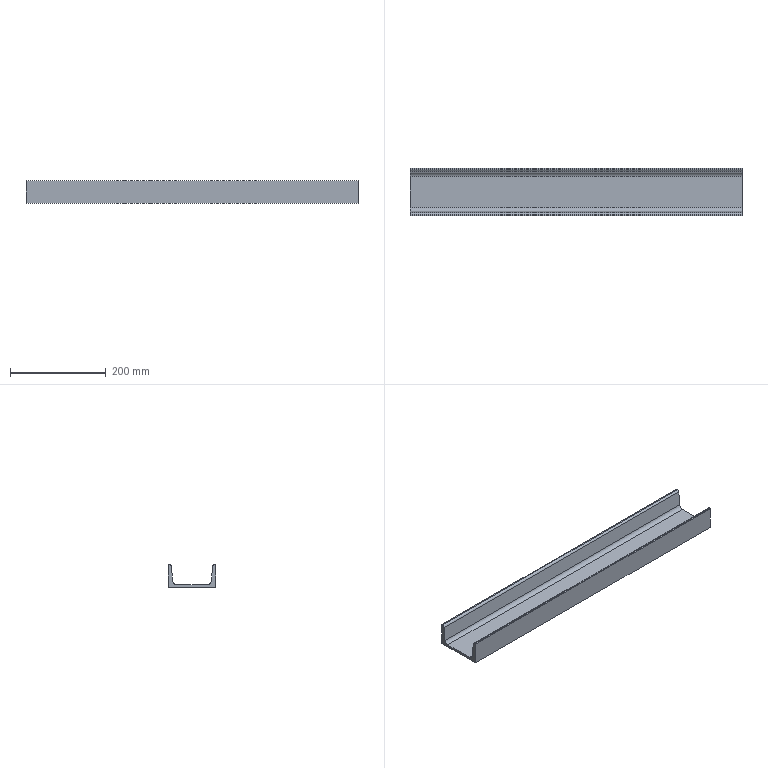Part | SolidWorks | features Fillet 2, Extrusion 1 | 1 solid | 14 faces | box 695 x 100 x 48 mm | volume 885612 mm3 | plane 10 | cylinder 4 | commonest cylinder face diameters 8.5 x2 17 x2
STEP:
#1=CARTESIAN_POINT('',(695.,43.252,44.173));
#2=VERTEX_POINT('',#1);
#3=CARTESIAN_POINT('',(695.,40.13,12.954));
#4=VERTEX_POINT('',#3);
#5=CARTESIAN_POINT('',(695.,39.365,5.3));
#6=DIRECTION('',(0.,-0.0995,-0.995));
#7=VECTOR('',#6,1000.);
#8=LINE('',#5,#7);
#9=EDGE_CURVE('',#2,#4,#8,.T.);
#10=ORIENTED_EDGE('',*,*,#9,.F.);
#11=CARTESIAN_POINT('',(0.,43.252,44.173));
#12=VERTEX_POINT('',#11);
#13=CARTESIAN_POINT('',(695.,43.252,44.173));
#14=DIRECTION('',(-1.,0.,0.));
#15=VECTOR('',#14,1000.);
#16=LINE('',#13,#15);
#17=EDGE_CURVE('',#2,#12,#16,.T.);
#18=ORIENTED_EDGE('',*,*,#17,.T.);
#19=CARTESIAN_POINT('',(0.,40.13,12.954));
#20=VERTEX_POINT('',#19);
#21=CARTESIAN_POINT('',(0.,39.365,5.3));
#22=DIRECTION('',(0.,-0.0995,-0.995));
#23=VECTOR('',#22,1000.);
#24=LINE('',#21,#23);
#25=EDGE_CURVE('',#12,#20,#24,.T.);
#26=ORIENTED_EDGE('',*,*,#25,.T.);
#27=CARTESIAN_POINT('',(695.,40.13,12.954));
#28=DIRECTION('',(1.,0.,0.));
#29=VECTOR('',#28,1000.);
#30=LINE('',#27,#29);
#31=EDGE_CURVE('',#20,#4,#30,.T.);
#32=ORIENTED_EDGE('',*,*,#31,.T.);
#33=EDGE_LOOP('',(#10,#18,#26,#32));
#34=FACE_OUTER_BOUND('',#33,.T.);
#35=CARTESIAN_POINT('',(695.,39.365,5.3));
#36=DIRECTION('',(0.,0.995,-0.0995));
#37=DIRECTION('',(0.,0.0995,0.995));
#38=AXIS2_PLACEMENT_3D('',#35,#36,#37);
#39=PLANE('',#38);
#40=ADVANCED_FACE('',(#34),#39,.F.);
#41=CARTESIAN_POINT('',(0.,31.673,5.3));
#42=VERTEX_POINT('',#41);
#43=CARTESIAN_POINT('',(0.,-31.673,5.3));
#44=VERTEX_POINT('',#43);
#45=CARTESIAN_POINT('',(0.,-39.365,5.3));
#46=DIRECTION('',(0.,-1.,0.));
#47=VECTOR('',#46,1000.);
#48=LINE('',#45,#47);
#49=EDGE_CURVE('',#42,#44,#48,.T.);
#50=ORIENTED_EDGE('',*,*,#49,.T.);
#51=CARTESIAN_POINT('',(695.,-31.673,5.3));
#52=VERTEX_POINT('',#51);
#53=CARTESIAN_POINT('',(695.,-31.673,5.3));
#54=DIRECTION('',(1.,0.,0.));
#55=VECTOR('',#54,1000.);
#56=LINE('',#53,#55);
#57=EDGE_CURVE('',#44,#52,#56,.T.);
#58=ORIENTED_EDGE('',*,*,#57,.T.);
#59=CARTESIAN_POINT('',(695.,31.673,5.3));
#60=VERTEX_POINT('',#59);
#61=CARTESIAN_POINT('',(695.,-39.365,5.3));
#62=DIRECTION('',(0.,-1.,0.));
#63=VECTOR('',#62,1000.);
#64=LINE('',#61,#63);
#65=EDGE_CURVE('',#60,#52,#64,.T.);
#66=ORIENTED_EDGE('',*,*,#65,.F.);
#67=CARTESIAN_POINT('',(0.,31.673,5.3));
#68=DIRECTION('',(-1.,0.,0.));
#69=VECTOR('',#68,1000.);
#70=LINE('',#67,#69);
#71=EDGE_CURVE('',#60,#42,#70,.T.);
#72=ORIENTED_EDGE('',*,*,#71,.T.);
#73=EDGE_LOOP('',(#50,#58,#66,#72));
#74=FACE_OUTER_BOUND('',#73,.T.);
#75=CARTESIAN_POINT('',(695.,-39.365,5.3));
#76=DIRECTION('',(0.,0.,-1.));
#77=DIRECTION('',(-1.,0.,0.));
#78=AXIS2_PLACEMENT_3D('',#75,#76,#77);
#79=PLANE('',#78);
#80=ADVANCED_FACE('',(#74),#79,.F.);
#81=CARTESIAN_POINT('',(0.,-40.13,12.954));
#82=VERTEX_POINT('',#81);
#83=CARTESIAN_POINT('',(0.,-43.252,44.173));
#84=VERTEX_POINT('',#83);
#85=CARTESIAN_POINT('',(0.,-39.365,5.3));
#86=DIRECTION('',(0.,-0.0995,0.995));
#87=VECTOR('',#86,1000.);
#88=LINE('',#85,#87);
#89=EDGE_CURVE('',#82,#84,#88,.T.);
#90=ORIENTED_EDGE('',*,*,#89,.T.);
#91=CARTESIAN_POINT('',(695.,-43.252,44.173));
#92=VERTEX_POINT('',#91);
#93=CARTESIAN_POINT('',(695.,-43.252,44.173));
#94=DIRECTION('',(1.,0.,0.));
#95=VECTOR('',#94,1000.);
#96=LINE('',#93,#95);
#97=EDGE_CURVE('',#84,#92,#96,.T.);
#98=ORIENTED_EDGE('',*,*,#97,.T.);
#99=CARTESIAN_POINT('',(695.,-40.13,12.954));
#100=VERTEX_POINT('',#99);
#101=CARTESIAN_POINT('',(695.,-39.365,5.3));
#102=DIRECTION('',(0.,-0.0995,0.995));
#103=VECTOR('',#102,1000.);
#104=LINE('',#101,#103);
#105=EDGE_CURVE('',#100,#92,#104,.T.);
#106=ORIENTED_EDGE('',*,*,#105,.F.);
#107=CARTESIAN_POINT('',(0.,-40.13,12.954));
#108=DIRECTION('',(-1.,0.,0.));
#109=VECTOR('',#108,1000.);
#110=LINE('',#107,#109);
#111=EDGE_CURVE('',#100,#82,#110,.T.);
#112=ORIENTED_EDGE('',*,*,#111,.T.);
#113=EDGE_LOOP('',(#90,#98,#106,#112));
#114=FACE_OUTER_BOUND('',#113,.T.);
#115=CARTESIAN_POINT('',(695.,-39.365,5.3));
#116=DIRECTION('',(0.,-0.995,-0.0995));
#117=DIRECTION('',(0.,0.0995,-0.995));
#118=AXIS2_PLACEMENT_3D('',#115,#116,#117);
#119=PLANE('',#118);
#120=ADVANCED_FACE('',(#114),#119,.F.);
#121=CARTESIAN_POINT('',(695.,-47.481,48.));
#122=VERTEX_POINT('',#121);
#123=CARTESIAN_POINT('',(695.,-50.,48.));
#124=VERTEX_POINT('',#123);
#125=CARTESIAN_POINT('',(695.,-43.635,48.));
#126=DIRECTION('',(0.,-1.,0.));
#127=VECTOR('',#126,1000.);
#128=LINE('',#125,#127);
#129=EDGE_CURVE('',#122,#124,#128,.T.);
#130=ORIENTED_EDGE('',*,*,#129,.F.);
#131=CARTESIAN_POINT('',(0.,-47.481,48.));
#132=VERTEX_POINT('',#131);
#133=CARTESIAN_POINT('',(695.,-47.481,48.));
#134=DIRECTION('',(-1.,0.,0.));
#135=VECTOR('',#134,1000.);
#136=LINE('',#133,#135);
#137=EDGE_CURVE('',#122,#132,#136,.T.);
#138=ORIENTED_EDGE('',*,*,#137,.T.);
#139=CARTESIAN_POINT('',(0.,-50.,48.));
#140=VERTEX_POINT('',#139);
#141=CARTESIAN_POINT('',(0.,-43.635,48.));
#142=DIRECTION('',(0.,-1.,0.));
#143=VECTOR('',#142,1000.);
#144=LINE('',#141,#143);
#145=EDGE_CURVE('',#132,#140,#144,.T.);
#146=ORIENTED_EDGE('',*,*,#145,.T.);
#147=CARTESIAN_POINT('',(695.,-50.,48.));
#148=DIRECTION('',(-1.,0.,0.));
#149=VECTOR('',#148,1000.);
#150=LINE('',#147,#149);
#151=EDGE_CURVE('',#124,#140,#150,.T.);
#152=ORIENTED_EDGE('',*,*,#151,.F.);
#153=EDGE_LOOP('',(#130,#138,#146,#152));
#154=FACE_OUTER_BOUND('',#153,.T.);
#155=CARTESIAN_POINT('',(695.,-43.635,48.));
#156=DIRECTION('',(0.,0.,-1.));
#157=DIRECTION('',(-1.,0.,0.));
#158=AXIS2_PLACEMENT_3D('',#155,#156,#157);
#159=PLANE('',#158);
#160=ADVANCED_FACE('',(#154),#159,.F.);
#161=CARTESIAN_POINT('',(0.,-50.,0.));
#162=VERTEX_POINT('',#161);
#163=CARTESIAN_POINT('',(0.,-50.,0.));
#164=DIRECTION('',(0.,0.,-1.));
#165=VECTOR('',#164,1000.);
#166=LINE('',#163,#165);
#167=EDGE_CURVE('',#140,#162,#166,.T.);
#168=ORIENTED_EDGE('',*,*,#167,.T.);
#169=CARTESIAN_POINT('',(695.,-50.,0.));
#170=VERTEX_POINT('',#169);
#171=CARTESIAN_POINT('',(695.,-50.,0.));
#172=DIRECTION('',(-1.,0.,0.));
#173=VECTOR('',#172,1000.);
#174=LINE('',#171,#173);
#175=EDGE_CURVE('',#170,#162,#174,.T.);
#176=ORIENTED_EDGE('',*,*,#175,.F.);
#177=CARTESIAN_POINT('',(695.,-50.,0.));
#178=DIRECTION('',(0.,0.,-1.));
#179=VECTOR('',#178,1000.);
#180=LINE('',#177,#179);
#181=EDGE_CURVE('',#124,#170,#180,.T.);
#182=ORIENTED_EDGE('',*,*,#181,.F.);
#183=ORIENTED_EDGE('',*,*,#151,.T.);
#184=EDGE_LOOP('',(#168,#176,#182,#183));
#185=FACE_OUTER_BOUND('',#184,.T.);
#186=CARTESIAN_POINT('',(695.,-50.,0.));
#187=DIRECTION('',(0.,1.,0.));
#188=DIRECTION('',(0.,0.,1.));
#189=AXIS2_PLACEMENT_3D('',#186,#187,#188);
#190=PLANE('',#189);
#191=ADVANCED_FACE('',(#185),#190,.F.);
#192=CARTESIAN_POINT('',(0.,50.,0.));
#193=VERTEX_POINT('',#192);
#194=CARTESIAN_POINT('',(0.,50.,0.));
#195=DIRECTION('',(0.,1.,0.));
#196=VECTOR('',#195,1000.);
#197=LINE('',#194,#196);
#198=EDGE_CURVE('',#162,#193,#197,.T.);
#199=ORIENTED_EDGE('',*,*,#198,.T.);
#200=CARTESIAN_POINT('',(695.,50.,0.));
#201=VERTEX_POINT('',#200);
#202=CARTESIAN_POINT('',(695.,50.,0.));
#203=DIRECTION('',(-1.,0.,0.));
#204=VECTOR('',#203,1000.);
#205=LINE('',#202,#204);
#206=EDGE_CURVE('',#201,#193,#205,.T.);
#207=ORIENTED_EDGE('',*,*,#206,.F.);
#208=CARTESIAN_POINT('',(695.,50.,0.));
#209=DIRECTION('',(0.,1.,0.));
#210=VECTOR('',#209,1000.);
#211=LINE('',#208,#210);
#212=EDGE_CURVE('',#170,#201,#211,.T.);
#213=ORIENTED_EDGE('',*,*,#212,.F.);
#214=ORIENTED_EDGE('',*,*,#175,.T.);
#215=EDGE_LOOP('',(#199,#207,#213,#214));
#216=FACE_OUTER_BOUND('',#215,.T.);
#217=CARTESIAN_POINT('',(695.,50.,0.));
#218=DIRECTION('',(0.,0.,1.));
#219=DIRECTION('',(0.,-1.,0.));
#220=AXIS2_PLACEMENT_3D('',#217,#218,#219);
#221=PLANE('',#220);
#222=ADVANCED_FACE('',(#216),#221,.F.);
#223=CARTESIAN_POINT('',(0.,50.,48.));
#224=VERTEX_POINT('',#223);
#225=CARTESIAN_POINT('',(0.,50.,0.));
#226=DIRECTION('',(0.,0.,1.));
#227=VECTOR('',#226,1000.);
#228=LINE('',#225,#227);
#229=EDGE_CURVE('',#193,#224,#228,.T.);
#230=ORIENTED_EDGE('',*,*,#229,.T.);
#231=CARTESIAN_POINT('',(695.,50.,48.));
#232=VERTEX_POINT('',#231);
#233=CARTESIAN_POINT('',(695.,50.,48.));
#234=DIRECTION('',(-1.,0.,0.));
#235=VECTOR('',#234,1000.);
#236=LINE('',#233,#235);
#237=EDGE_CURVE('',#232,#224,#236,.T.);
#238=ORIENTED_EDGE('',*,*,#237,.F.);
#239=CARTESIAN_POINT('',(695.,50.,0.));
#240=DIRECTION('',(0.,0.,1.));
#241=VECTOR('',#240,1000.);
#242=LINE('',#239,#241);
#243=EDGE_CURVE('',#201,#232,#242,.T.);
#244=ORIENTED_EDGE('',*,*,#243,.F.);
#245=ORIENTED_EDGE('',*,*,#206,.T.);
#246=EDGE_LOOP('',(#230,#238,#244,#245));
#247=FACE_OUTER_BOUND('',#246,.T.);
#248=CARTESIAN_POINT('',(695.,50.,0.));
#249=DIRECTION('',(0.,-1.,0.));
#250=DIRECTION('',(0.,0.,-1.));
#251=AXIS2_PLACEMENT_3D('',#248,#249,#250);
#252=PLANE('',#251);
#253=ADVANCED_FACE('',(#247),#252,.F.);
#254=CARTESIAN_POINT('',(0.,47.481,48.));
#255=VERTEX_POINT('',#254);
#256=CARTESIAN_POINT('',(0.,43.635,48.));
#257=DIRECTION('',(0.,-1.,0.));
#258=VECTOR('',#257,1000.);
#259=LINE('',#256,#258);
#260=EDGE_CURVE('',#224,#255,#259,.T.);
#261=ORIENTED_EDGE('',*,*,#260,.T.);
#262=CARTESIAN_POINT('',(695.,47.481,48.));
#263=VERTEX_POINT('',#262);
#264=CARTESIAN_POINT('',(695.,47.481,48.));
#265=DIRECTION('',(1.,0.,0.));
#266=VECTOR('',#265,1000.);
#267=LINE('',#264,#266);
#268=EDGE_CURVE('',#255,#263,#267,.T.);
#269=ORIENTED_EDGE('',*,*,#268,.T.);
#270=CARTESIAN_POINT('',(695.,43.635,48.));
#271=DIRECTION('',(0.,-1.,0.));
#272=VECTOR('',#271,1000.);
#273=LINE('',#270,#272);
#274=EDGE_CURVE('',#232,#263,#273,.T.);
#275=ORIENTED_EDGE('',*,*,#274,.F.);
#276=ORIENTED_EDGE('',*,*,#237,.T.);
#277=EDGE_LOOP('',(#261,#269,#275,#276));
#278=FACE_OUTER_BOUND('',#277,.T.);
#279=CARTESIAN_POINT('',(695.,43.635,48.));
#280=DIRECTION('',(0.,0.,-1.));
#281=DIRECTION('',(-1.,0.,0.));
#282=AXIS2_PLACEMENT_3D('',#279,#280,#281);
#283=PLANE('',#282);
#284=ADVANCED_FACE('',(#278),#283,.F.);
#285=ORIENTED_EDGE('',*,*,#105,.T.);
#286=CARTESIAN_POINT('',(695.,-47.481,43.75));
#287=DIRECTION('',(1.,0.,0.));
#288=DIRECTION('',(0.,0.,-1.));
#289=AXIS2_PLACEMENT_3D('',#286,#287,#288);
#290=CIRCLE('',#289,4.25);
#291=EDGE_CURVE('',#92,#122,#290,.T.);
#292=ORIENTED_EDGE('',*,*,#291,.T.);
#293=ORIENTED_EDGE('',*,*,#129,.T.);
#294=ORIENTED_EDGE('',*,*,#181,.T.);
#295=ORIENTED_EDGE('',*,*,#212,.T.);
#296=ORIENTED_EDGE('',*,*,#243,.T.);
#297=ORIENTED_EDGE('',*,*,#274,.T.);
#298=CARTESIAN_POINT('',(695.,47.481,43.75));
#299=DIRECTION('',(1.,0.,0.));
#300=DIRECTION('',(0.,0.,-1.));
#301=AXIS2_PLACEMENT_3D('',#298,#299,#300);
#302=CIRCLE('',#301,4.25);
#303=EDGE_CURVE('',#263,#2,#302,.T.);
#304=ORIENTED_EDGE('',*,*,#303,.T.);
#305=ORIENTED_EDGE('',*,*,#9,.T.);
#306=CARTESIAN_POINT('',(695.,31.673,13.8));
#307=DIRECTION('',(-1.,0.,0.));
#308=DIRECTION('',(0.,0.,-1.));
#309=AXIS2_PLACEMENT_3D('',#306,#307,#308);
#310=CIRCLE('',#309,8.5);
#311=EDGE_CURVE('',#4,#60,#310,.T.);
#312=ORIENTED_EDGE('',*,*,#311,.T.);
#313=ORIENTED_EDGE('',*,*,#65,.T.);
#314=CARTESIAN_POINT('',(695.,-31.673,13.8));
#315=DIRECTION('',(-1.,0.,0.));
#316=DIRECTION('',(0.,0.,-1.));
#317=AXIS2_PLACEMENT_3D('',#314,#315,#316);
#318=CIRCLE('',#317,8.5);
#319=EDGE_CURVE('',#52,#100,#318,.T.);
#320=ORIENTED_EDGE('',*,*,#319,.T.);
#321=EDGE_LOOP('',(#285,#292,#293,#294,#295,#296,#297,#304,#305,#312,#313,#320));
#322=FACE_OUTER_BOUND('',#321,.T.);
#323=CARTESIAN_POINT('',(695.,38.835,0.));
#324=DIRECTION('',(1.,0.,0.));
#325=DIRECTION('',(0.,0.,-1.));
#326=AXIS2_PLACEMENT_3D('',#323,#324,#325);
#327=PLANE('',#326);
#328=ADVANCED_FACE('',(#322),#327,.T.);
#329=ORIENTED_EDGE('',*,*,#145,.F.);
#330=CARTESIAN_POINT('',(0.,-47.481,43.75));
#331=DIRECTION('',(-1.,0.,0.));
#332=DIRECTION('',(0.,0.,-1.));
#333=AXIS2_PLACEMENT_3D('',#330,#331,#332);
#334=CIRCLE('',#333,4.25);
#335=EDGE_CURVE('',#132,#84,#334,.T.);
#336=ORIENTED_EDGE('',*,*,#335,.T.);
#337=ORIENTED_EDGE('',*,*,#89,.F.);
#338=CARTESIAN_POINT('',(0.,-31.673,13.8));
#339=DIRECTION('',(1.,0.,0.));
#340=DIRECTION('',(0.,0.,-1.));
#341=AXIS2_PLACEMENT_3D('',#338,#339,#340);
#342=CIRCLE('',#341,8.5);
#343=EDGE_CURVE('',#82,#44,#342,.T.);
#344=ORIENTED_EDGE('',*,*,#343,.T.);
#345=ORIENTED_EDGE('',*,*,#49,.F.);
#346=CARTESIAN_POINT('',(0.,31.673,13.8));
#347=DIRECTION('',(1.,0.,0.));
#348=DIRECTION('',(0.,0.,-1.));
#349=AXIS2_PLACEMENT_3D('',#346,#347,#348);
#350=CIRCLE('',#349,8.5);
#351=EDGE_CURVE('',#42,#20,#350,.T.);
#352=ORIENTED_EDGE('',*,*,#351,.T.);
#353=ORIENTED_EDGE('',*,*,#25,.F.);
#354=CARTESIAN_POINT('',(0.,47.481,43.75));
#355=DIRECTION('',(-1.,0.,0.));
#356=DIRECTION('',(0.,0.,-1.));
#357=AXIS2_PLACEMENT_3D('',#354,#355,#356);
#358=CIRCLE('',#357,4.25);
#359=EDGE_CURVE('',#12,#255,#358,.T.);
#360=ORIENTED_EDGE('',*,*,#359,.T.);
#361=ORIENTED_EDGE('',*,*,#260,.F.);
#362=ORIENTED_EDGE('',*,*,#229,.F.);
#363=ORIENTED_EDGE('',*,*,#198,.F.);
#364=ORIENTED_EDGE('',*,*,#167,.F.);
#365=EDGE_LOOP('',(#329,#336,#337,#344,#345,#352,#353,#360,#361,#362,#363,#364));
#366=FACE_OUTER_BOUND('',#365,.T.);
#367=CARTESIAN_POINT('',(0.,38.835,0.));
#368=DIRECTION('',(1.,0.,0.));
#369=DIRECTION('',(0.,0.,-1.));
#370=AXIS2_PLACEMENT_3D('',#367,#368,#369);
#371=PLANE('',#370);
#372=ADVANCED_FACE('',(#366),#371,.F.);
#373=ORIENTED_EDGE('',*,*,#319,.F.);
#374=ORIENTED_EDGE('',*,*,#57,.F.);
#375=ORIENTED_EDGE('',*,*,#343,.F.);
#376=ORIENTED_EDGE('',*,*,#111,.F.);
#377=EDGE_LOOP('',(#373,#374,#375,#376));
#378=FACE_OUTER_BOUND('',#377,.T.);
#379=CARTESIAN_POINT('',(695.,-31.673,13.8));
#380=DIRECTION('',(1.,0.,0.));
#381=DIRECTION('',(0.,0.,-1.));
#382=AXIS2_PLACEMENT_3D('',#379,#380,#381);
#383=CYLINDRICAL_SURFACE('',#382,8.5);
#384=ADVANCED_FACE('',(#378),#383,.F.);
#385=ORIENTED_EDGE('',*,*,#311,.F.);
#386=ORIENTED_EDGE('',*,*,#31,.F.);
#387=ORIENTED_EDGE('',*,*,#351,.F.);
#388=ORIENTED_EDGE('',*,*,#71,.F.);
#389=EDGE_LOOP('',(#385,#386,#387,#388));
#390=FACE_OUTER_BOUND('',#389,.T.);
#391=CARTESIAN_POINT('',(695.,31.673,13.8));
#392=DIRECTION('',(1.,0.,0.));
#393=DIRECTION('',(0.,0.,-1.));
#394=AXIS2_PLACEMENT_3D('',#391,#392,#393);
#395=CYLINDRICAL_SURFACE('',#394,8.5);
#396=ADVANCED_FACE('',(#390),#395,.F.);
#397=ORIENTED_EDGE('',*,*,#291,.F.);
#398=ORIENTED_EDGE('',*,*,#97,.F.);
#399=ORIENTED_EDGE('',*,*,#335,.F.);
#400=ORIENTED_EDGE('',*,*,#137,.F.);
#401=EDGE_LOOP('',(#397,#398,#399,#400));
#402=FACE_OUTER_BOUND('',#401,.T.);
#403=CARTESIAN_POINT('',(695.,-47.481,43.75));
#404=DIRECTION('',(-1.,0.,0.));
#405=DIRECTION('',(0.,0.,1.));
#406=AXIS2_PLACEMENT_3D('',#403,#404,#405);
#407=CYLINDRICAL_SURFACE('',#406,4.25);
#408=ADVANCED_FACE('',(#402),#407,.T.);
#409=ORIENTED_EDGE('',*,*,#303,.F.);
#410=ORIENTED_EDGE('',*,*,#268,.F.);
#411=ORIENTED_EDGE('',*,*,#359,.F.);
#412=ORIENTED_EDGE('',*,*,#17,.F.);
#413=EDGE_LOOP('',(#409,#410,#411,#412));
#414=FACE_OUTER_BOUND('',#413,.T.);
#415=CARTESIAN_POINT('',(695.,47.481,43.75));
#416=DIRECTION('',(-1.,0.,0.));
#417=DIRECTION('',(0.,0.,1.));
#418=AXIS2_PLACEMENT_3D('',#415,#416,#417);
#419=CYLINDRICAL_SURFACE('',#418,4.25);
#420=ADVANCED_FACE('',(#414),#419,.T.);
#421=CLOSED_SHELL('',(#40,#80,#120,#160,#191,#222,#253,#284,#328,#372,#384,#396,#408,#420));
#422=MANIFOLD_SOLID_BREP('',#421);
#423=CARTESIAN_POINT('',(0.,0.,0.));
#424=DIRECTION('',(0.,0.,1.));
#425=DIRECTION('',(1.,0.,0.));
#426=AXIS2_PLACEMENT_3D('',#423,#424,#425);
#427=(LENGTH_UNIT()NAMED_UNIT(*)SI_UNIT(.MILLI.,.METRE.));
#428=UNCERTAINTY_MEASURE_WITH_UNIT(LENGTH_MEASURE(0.00001),#427,'','');
#429=(NAMED_UNIT(*)PLANE_ANGLE_UNIT()SI_UNIT($,.RADIAN.));
#430=(NAMED_UNIT(*)SI_UNIT($,.STERADIAN.)SOLID_ANGLE_UNIT());
#431=(GEOMETRIC_REPRESENTATION_CONTEXT(3)GLOBAL_UNCERTAINTY_ASSIGNED_CONTEXT((#428))GLOBAL_UNIT_ASSIGNED_CONTEXT((#427,#429,#430))REPRESENTATION_CONTEXT('',''));
#432=ADVANCED_BREP_SHAPE_REPRESENTATION('',(#422,#426),#431);